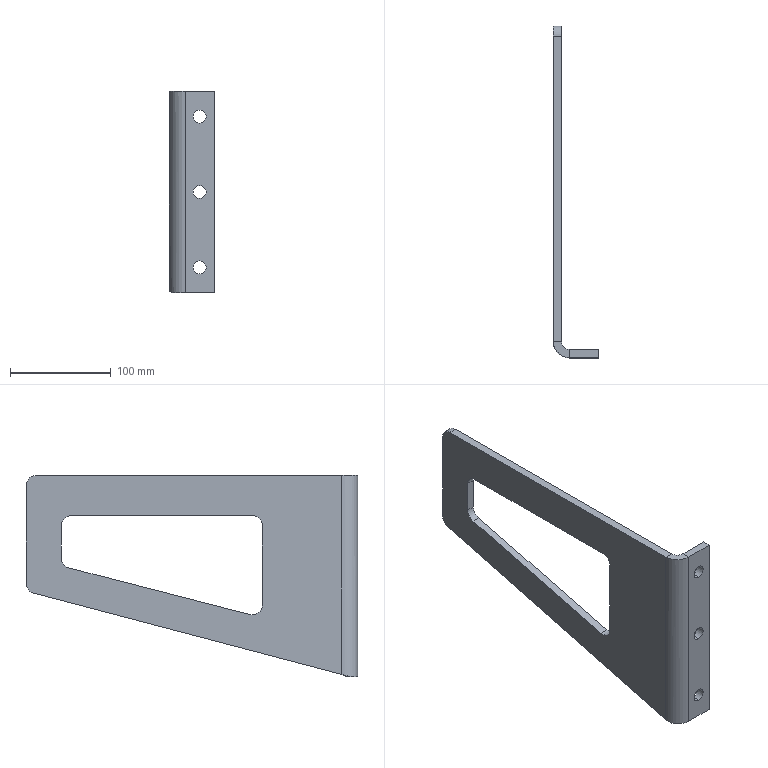Part | SolidWorks | features ICE 2, FlatPattern 1, SMBaseFlange 1, SheetMetal 1 | 1 solid | 31 faces | box 45 x 330 x 200 mm | volume 345586 mm3 | plane 16 | cylinder 14 | spline 1 | commonest cylinder face diameters 13 x6 20 x6 16 x1 32 x1
STEP:
#1=CARTESIAN_POINT('',(-3.464,-55.999,-168.5));
#2=VERTEX_POINT('',#1);
#3=CARTESIAN_POINT('',(-3.464,-55.999,-181.5));
#4=VERTEX_POINT('',#3);
#5=CARTESIAN_POINT('',(-3.464,-55.999,-175.));
#6=DIRECTION('',(0.,-1.,0.));
#7=DIRECTION('',(0.,0.,-1.));
#8=AXIS2_PLACEMENT_3D('',#5,#6,#7);
#9=CIRCLE('',#8,6.5);
#10=EDGE_CURVE('',#2,#4,#9,.T.);
#11=ORIENTED_EDGE('',*,*,#10,.F.);
#12=CARTESIAN_POINT('',(-3.464,-63.999,-168.5));
#13=VERTEX_POINT('',#12);
#14=CARTESIAN_POINT('',(-3.464,266.001,-168.5));
#15=DIRECTION('',(0.,-1.,0.));
#16=VECTOR('',#15,1000.);
#17=LINE('',#14,#16);
#18=EDGE_CURVE('',#2,#13,#17,.T.);
#19=ORIENTED_EDGE('',*,*,#18,.T.);
#20=CARTESIAN_POINT('',(-3.464,-63.999,-181.5));
#21=VERTEX_POINT('',#20);
#22=CARTESIAN_POINT('',(-3.464,-63.999,-175.));
#23=DIRECTION('',(0.,-1.,0.));
#24=DIRECTION('',(0.,0.,-1.));
#25=AXIS2_PLACEMENT_3D('',#22,#23,#24);
#26=CIRCLE('',#25,6.5);
#27=EDGE_CURVE('',#13,#21,#26,.T.);
#28=ORIENTED_EDGE('',*,*,#27,.T.);
#29=CARTESIAN_POINT('',(-3.464,266.001,-181.5));
#30=DIRECTION('',(0.,-1.,0.));
#31=VECTOR('',#30,1000.);
#32=LINE('',#29,#31);
#33=EDGE_CURVE('',#4,#21,#32,.T.);
#34=ORIENTED_EDGE('',*,*,#33,.F.);
#35=EDGE_LOOP('',(#11,#19,#28,#34));
#36=FACE_OUTER_BOUND('',#35,.T.);
#37=CARTESIAN_POINT('',(-3.464,266.001,-175.));
#38=DIRECTION('',(0.,-1.,0.));
#39=DIRECTION('',(0.,0.,-1.));
#40=AXIS2_PLACEMENT_3D('',#37,#38,#39);
#41=CYLINDRICAL_SURFACE('',#40,6.5);
#42=ADVANCED_FACE('',(#36),#41,.F.);
#43=CARTESIAN_POINT('',(-3.464,-55.999,-93.5));
#44=VERTEX_POINT('',#43);
#45=CARTESIAN_POINT('',(-3.464,-55.999,-106.5));
#46=VERTEX_POINT('',#45);
#47=CARTESIAN_POINT('',(-3.464,-55.999,-100.));
#48=DIRECTION('',(0.,-1.,0.));
#49=DIRECTION('',(0.,0.,-1.));
#50=AXIS2_PLACEMENT_3D('',#47,#48,#49);
#51=CIRCLE('',#50,6.5);
#52=EDGE_CURVE('',#44,#46,#51,.T.);
#53=ORIENTED_EDGE('',*,*,#52,.F.);
#54=CARTESIAN_POINT('',(-3.464,-63.999,-93.5));
#55=VERTEX_POINT('',#54);
#56=CARTESIAN_POINT('',(-3.464,266.001,-93.5));
#57=DIRECTION('',(0.,-1.,0.));
#58=VECTOR('',#57,1000.);
#59=LINE('',#56,#58);
#60=EDGE_CURVE('',#44,#55,#59,.T.);
#61=ORIENTED_EDGE('',*,*,#60,.T.);
#62=CARTESIAN_POINT('',(-3.464,-63.999,-106.5));
#63=VERTEX_POINT('',#62);
#64=CARTESIAN_POINT('',(-3.464,-63.999,-100.));
#65=DIRECTION('',(0.,-1.,0.));
#66=DIRECTION('',(0.,0.,-1.));
#67=AXIS2_PLACEMENT_3D('',#64,#65,#66);
#68=CIRCLE('',#67,6.5);
#69=EDGE_CURVE('',#55,#63,#68,.T.);
#70=ORIENTED_EDGE('',*,*,#69,.T.);
#71=CARTESIAN_POINT('',(-3.464,266.001,-106.5));
#72=DIRECTION('',(0.,-1.,0.));
#73=VECTOR('',#72,1000.);
#74=LINE('',#71,#73);
#75=EDGE_CURVE('',#46,#63,#74,.T.);
#76=ORIENTED_EDGE('',*,*,#75,.F.);
#77=EDGE_LOOP('',(#53,#61,#70,#76));
#78=FACE_OUTER_BOUND('',#77,.T.);
#79=CARTESIAN_POINT('',(-3.464,266.001,-100.));
#80=DIRECTION('',(0.,-1.,0.));
#81=DIRECTION('',(0.,0.,-1.));
#82=AXIS2_PLACEMENT_3D('',#79,#80,#81);
#83=CYLINDRICAL_SURFACE('',#82,6.5);
#84=ADVANCED_FACE('',(#78),#83,.F.);
#85=CARTESIAN_POINT('',(-3.465,-55.999,-18.5));
#86=VERTEX_POINT('',#85);
#87=CARTESIAN_POINT('',(-3.465,-55.999,-31.5));
#88=VERTEX_POINT('',#87);
#89=CARTESIAN_POINT('',(-3.465,-55.999,-25.));
#90=DIRECTION('',(0.,-1.,0.));
#91=DIRECTION('',(0.,0.,-1.));
#92=AXIS2_PLACEMENT_3D('',#89,#90,#91);
#93=CIRCLE('',#92,6.5);
#94=EDGE_CURVE('',#86,#88,#93,.T.);
#95=ORIENTED_EDGE('',*,*,#94,.F.);
#96=CARTESIAN_POINT('',(-3.465,-63.999,-18.5));
#97=VERTEX_POINT('',#96);
#98=CARTESIAN_POINT('',(-3.465,266.001,-18.5));
#99=DIRECTION('',(0.,-1.,0.));
#100=VECTOR('',#99,1000.);
#101=LINE('',#98,#100);
#102=EDGE_CURVE('',#86,#97,#101,.T.);
#103=ORIENTED_EDGE('',*,*,#102,.T.);
#104=CARTESIAN_POINT('',(-3.465,-63.999,-31.5));
#105=VERTEX_POINT('',#104);
#106=CARTESIAN_POINT('',(-3.465,-63.999,-25.));
#107=DIRECTION('',(0.,-1.,0.));
#108=DIRECTION('',(0.,0.,-1.));
#109=AXIS2_PLACEMENT_3D('',#106,#107,#108);
#110=CIRCLE('',#109,6.5);
#111=EDGE_CURVE('',#97,#105,#110,.T.);
#112=ORIENTED_EDGE('',*,*,#111,.T.);
#113=CARTESIAN_POINT('',(-3.465,266.001,-31.5));
#114=DIRECTION('',(0.,-1.,0.));
#115=VECTOR('',#114,1000.);
#116=LINE('',#113,#115);
#117=EDGE_CURVE('',#88,#105,#116,.T.);
#118=ORIENTED_EDGE('',*,*,#117,.F.);
#119=EDGE_LOOP('',(#95,#103,#112,#118));
#120=FACE_OUTER_BOUND('',#119,.T.);
#121=CARTESIAN_POINT('',(-3.465,266.001,-25.));
#122=DIRECTION('',(0.,-1.,0.));
#123=DIRECTION('',(0.,0.,-1.));
#124=AXIS2_PLACEMENT_3D('',#121,#122,#123);
#125=CYLINDRICAL_SURFACE('',#124,6.5);
#126=ADVANCED_FACE('',(#120),#125,.F.);
#127=CARTESIAN_POINT('',(-33.465,43.495,-138.283));
#128=VERTEX_POINT('',#127);
#129=CARTESIAN_POINT('',(-33.465,223.495,-91.933));
#130=VERTEX_POINT('',#129);
#131=CARTESIAN_POINT('',(-33.465,43.495,-138.283));
#132=DIRECTION('',(0.,0.9684,0.2494));
#133=VECTOR('',#132,1000.);
#134=LINE('',#131,#133);
#135=EDGE_CURVE('',#128,#130,#134,.T.);
#136=ORIENTED_EDGE('',*,*,#135,.T.);
#137=CARTESIAN_POINT('',(-33.465,231.001,-82.249));
#138=VERTEX_POINT('',#137);
#139=CARTESIAN_POINT('',(-33.465,221.001,-82.249));
#140=DIRECTION('',(1.,0.,0.));
#141=DIRECTION('',(0.,1.,0.));
#142=AXIS2_PLACEMENT_3D('',#139,#140,#141);
#143=CIRCLE('',#142,10.);
#144=EDGE_CURVE('',#130,#138,#143,.T.);
#145=ORIENTED_EDGE('',*,*,#144,.T.);
#146=CARTESIAN_POINT('',(-33.465,231.001,-50.));
#147=VERTEX_POINT('',#146);
#148=CARTESIAN_POINT('',(-33.465,231.001,-200.));
#149=DIRECTION('',(0.,0.,1.));
#150=VECTOR('',#149,1000.);
#151=LINE('',#148,#150);
#152=EDGE_CURVE('',#138,#147,#151,.T.);
#153=ORIENTED_EDGE('',*,*,#152,.T.);
#154=CARTESIAN_POINT('',(-33.465,221.001,-40.));
#155=VERTEX_POINT('',#154);
#156=CARTESIAN_POINT('',(-33.465,221.001,-50.));
#157=DIRECTION('',(1.,0.,0.));
#158=DIRECTION('',(0.,1.,0.));
#159=AXIS2_PLACEMENT_3D('',#156,#157,#158);
#160=CIRCLE('',#159,10.);
#161=EDGE_CURVE('',#147,#155,#160,.T.);
#162=ORIENTED_EDGE('',*,*,#161,.T.);
#163=CARTESIAN_POINT('',(-33.465,41.001,-40.));
#164=VERTEX_POINT('',#163);
#165=CARTESIAN_POINT('',(-33.465,266.001,-40.));
#166=DIRECTION('',(0.,-1.,0.));
#167=VECTOR('',#166,1000.);
#168=LINE('',#165,#167);
#169=EDGE_CURVE('',#155,#164,#168,.T.);
#170=ORIENTED_EDGE('',*,*,#169,.T.);
#171=CARTESIAN_POINT('',(-33.465,31.001,-50.));
#172=VERTEX_POINT('',#171);
#173=CARTESIAN_POINT('',(-33.465,41.001,-50.));
#174=DIRECTION('',(1.,0.,0.));
#175=DIRECTION('',(0.,1.,0.));
#176=AXIS2_PLACEMENT_3D('',#173,#174,#175);
#177=CIRCLE('',#176,10.);
#178=EDGE_CURVE('',#164,#172,#177,.T.);
#179=ORIENTED_EDGE('',*,*,#178,.T.);
#180=CARTESIAN_POINT('',(-33.465,31.001,-128.599));
#181=VERTEX_POINT('',#180);
#182=CARTESIAN_POINT('',(-33.465,31.001,-200.));
#183=DIRECTION('',(0.,0.,-1.));
#184=VECTOR('',#183,1000.);
#185=LINE('',#182,#184);
#186=EDGE_CURVE('',#172,#181,#185,.T.);
#187=ORIENTED_EDGE('',*,*,#186,.T.);
#188=CARTESIAN_POINT('',(-33.465,41.001,-128.599));
#189=DIRECTION('',(1.,0.,0.));
#190=DIRECTION('',(0.,1.,0.));
#191=AXIS2_PLACEMENT_3D('',#188,#189,#190);
#192=CIRCLE('',#191,10.);
#193=EDGE_CURVE('',#181,#128,#192,.T.);
#194=ORIENTED_EDGE('',*,*,#193,.T.);
#195=EDGE_LOOP('',(#136,#145,#153,#162,#170,#179,#187,#194));
#196=FACE_BOUND('',#195,.T.);
#197=CARTESIAN_POINT('',(-33.465,266.001,-107.297));
#198=VERTEX_POINT('',#197);
#199=CARTESIAN_POINT('',(-33.465,266.001,-10.));
#200=VERTEX_POINT('',#199);
#201=CARTESIAN_POINT('',(-33.465,266.001,-200.));
#202=DIRECTION('',(0.,0.,1.));
#203=VECTOR('',#202,1000.);
#204=LINE('',#201,#203);
#205=EDGE_CURVE('',#198,#200,#204,.T.);
#206=ORIENTED_EDGE('',*,*,#205,.F.);
#207=CARTESIAN_POINT('',(-33.465,258.553,-116.966));
#208=VERTEX_POINT('',#207);
#209=CARTESIAN_POINT('',(-33.465,256.001,-107.297));
#210=DIRECTION('',(-1.,0.,0.));
#211=DIRECTION('',(0.,-1.,0.));
#212=AXIS2_PLACEMENT_3D('',#209,#210,#211);
#213=CIRCLE('',#212,10.);
#214=EDGE_CURVE('',#198,#208,#213,.T.);
#215=ORIENTED_EDGE('',*,*,#214,.T.);
#216=CARTESIAN_POINT('',(-33.465,-47.999,-197.888));
#217=VERTEX_POINT('',#216);
#218=CARTESIAN_POINT('',(-33.465,-55.999,-200.));
#219=DIRECTION('',(0.,-0.9669,-0.2552));
#220=VECTOR('',#219,1000.);
#221=LINE('',#218,#220);
#222=EDGE_CURVE('',#208,#217,#221,.T.);
#223=ORIENTED_EDGE('',*,*,#222,.T.);
#224=CARTESIAN_POINT('',(-33.465,-47.999,0.));
#225=VERTEX_POINT('',#224);
#226=CARTESIAN_POINT('',(-33.465,-47.999,-200.));
#227=DIRECTION('',(0.,0.,1.));
#228=VECTOR('',#227,1000.);
#229=LINE('',#226,#228);
#230=EDGE_CURVE('',#217,#225,#229,.T.);
#231=ORIENTED_EDGE('',*,*,#230,.T.);
#232=CARTESIAN_POINT('',(-33.465,256.001,0.));
#233=VERTEX_POINT('',#232);
#234=CARTESIAN_POINT('',(-33.465,266.001,0.));
#235=DIRECTION('',(0.,-1.,0.));
#236=VECTOR('',#235,1000.);
#237=LINE('',#234,#236);
#238=EDGE_CURVE('',#233,#225,#237,.T.);
#239=ORIENTED_EDGE('',*,*,#238,.F.);
#240=CARTESIAN_POINT('',(-33.465,256.001,-10.));
#241=DIRECTION('',(-1.,0.,0.));
#242=DIRECTION('',(0.,-1.,0.));
#243=AXIS2_PLACEMENT_3D('',#240,#241,#242);
#244=CIRCLE('',#243,10.);
#245=EDGE_CURVE('',#233,#200,#244,.T.);
#246=ORIENTED_EDGE('',*,*,#245,.T.);
#247=EDGE_LOOP('',(#206,#215,#223,#231,#239,#246));
#248=FACE_OUTER_BOUND('',#247,.T.);
#249=CARTESIAN_POINT('',(-33.465,266.001,-200.));
#250=DIRECTION('',(-1.,0.,0.));
#251=DIRECTION('',(0.,-1.,0.));
#252=AXIS2_PLACEMENT_3D('',#249,#250,#251);
#253=PLANE('',#252);
#254=ADVANCED_FACE('',(#196,#248),#253,.T.);
#255=CARTESIAN_POINT('',(-25.465,223.495,-91.933));
#256=VERTEX_POINT('',#255);
#257=CARTESIAN_POINT('',(-25.465,231.001,-82.249));
#258=VERTEX_POINT('',#257);
#259=CARTESIAN_POINT('',(-25.465,221.001,-82.249));
#260=DIRECTION('',(1.,0.,0.));
#261=DIRECTION('',(0.,1.,0.));
#262=AXIS2_PLACEMENT_3D('',#259,#260,#261);
#263=CIRCLE('',#262,10.);
#264=EDGE_CURVE('',#256,#258,#263,.T.);
#265=ORIENTED_EDGE('',*,*,#264,.F.);
#266=CARTESIAN_POINT('',(-25.465,43.495,-138.283));
#267=VERTEX_POINT('',#266);
#268=CARTESIAN_POINT('',(-25.465,43.495,-138.283));
#269=DIRECTION('',(0.,0.9684,0.2494));
#270=VECTOR('',#269,1000.);
#271=LINE('',#268,#270);
#272=EDGE_CURVE('',#267,#256,#271,.T.);
#273=ORIENTED_EDGE('',*,*,#272,.F.);
#274=CARTESIAN_POINT('',(-25.465,31.001,-128.599));
#275=VERTEX_POINT('',#274);
#276=CARTESIAN_POINT('',(-25.465,41.001,-128.599));
#277=DIRECTION('',(1.,0.,0.));
#278=DIRECTION('',(0.,-1.,0.));
#279=AXIS2_PLACEMENT_3D('',#276,#277,#278);
#280=CIRCLE('',#279,10.);
#281=EDGE_CURVE('',#275,#267,#280,.T.);
#282=ORIENTED_EDGE('',*,*,#281,.F.);
#283=CARTESIAN_POINT('',(-25.465,31.001,-50.));
#284=VERTEX_POINT('',#283);
#285=CARTESIAN_POINT('',(-25.465,31.001,-50.));
#286=DIRECTION('',(0.,0.,-1.));
#287=VECTOR('',#286,1000.);
#288=LINE('',#285,#287);
#289=EDGE_CURVE('',#284,#275,#288,.T.);
#290=ORIENTED_EDGE('',*,*,#289,.F.);
#291=CARTESIAN_POINT('',(-25.465,41.001,-40.));
#292=VERTEX_POINT('',#291);
#293=CARTESIAN_POINT('',(-25.465,41.001,-50.));
#294=DIRECTION('',(1.,0.,0.));
#295=DIRECTION('',(0.,1.,0.));
#296=AXIS2_PLACEMENT_3D('',#293,#294,#295);
#297=CIRCLE('',#296,10.);
#298=EDGE_CURVE('',#292,#284,#297,.T.);
#299=ORIENTED_EDGE('',*,*,#298,.F.);
#300=CARTESIAN_POINT('',(-25.465,221.001,-40.));
#301=VERTEX_POINT('',#300);
#302=CARTESIAN_POINT('',(-25.465,41.001,-40.));
#303=DIRECTION('',(0.,-1.,0.));
#304=VECTOR('',#303,1000.);
#305=LINE('',#302,#304);
#306=EDGE_CURVE('',#301,#292,#305,.T.);
#307=ORIENTED_EDGE('',*,*,#306,.F.);
#308=CARTESIAN_POINT('',(-25.465,231.001,-50.));
#309=VERTEX_POINT('',#308);
#310=CARTESIAN_POINT('',(-25.465,221.001,-50.));
#311=DIRECTION('',(1.,0.,0.));
#312=DIRECTION('',(0.,-1.,0.));
#313=AXIS2_PLACEMENT_3D('',#310,#311,#312);
#314=CIRCLE('',#313,10.);
#315=EDGE_CURVE('',#309,#301,#314,.T.);
#316=ORIENTED_EDGE('',*,*,#315,.F.);
#317=CARTESIAN_POINT('',(-25.465,231.001,-50.));
#318=DIRECTION('',(0.,0.,1.));
#319=VECTOR('',#318,1000.);
#320=LINE('',#317,#319);
#321=EDGE_CURVE('',#258,#309,#320,.T.);
#322=ORIENTED_EDGE('',*,*,#321,.F.);
#323=EDGE_LOOP('',(#265,#273,#282,#290,#299,#307,#316,#322));
#324=FACE_BOUND('',#323,.T.);
#325=CARTESIAN_POINT('',(-25.465,266.001,-107.297));
#326=VERTEX_POINT('',#325);
#327=CARTESIAN_POINT('',(-25.465,258.553,-116.966));
#328=VERTEX_POINT('',#327);
#329=CARTESIAN_POINT('',(-25.465,256.001,-107.297));
#330=DIRECTION('',(-1.,0.,0.));
#331=DIRECTION('',(0.,1.,0.));
#332=AXIS2_PLACEMENT_3D('',#329,#330,#331);
#333=CIRCLE('',#332,10.);
#334=EDGE_CURVE('',#326,#328,#333,.T.);
#335=ORIENTED_EDGE('',*,*,#334,.F.);
#336=CARTESIAN_POINT('',(-25.465,266.001,-10.));
#337=VERTEX_POINT('',#336);
#338=CARTESIAN_POINT('',(-25.465,266.001,-200.));
#339=DIRECTION('',(0.,0.,1.));
#340=VECTOR('',#339,1000.);
#341=LINE('',#338,#340);
#342=EDGE_CURVE('',#326,#337,#341,.T.);
#343=ORIENTED_EDGE('',*,*,#342,.T.);
#344=CARTESIAN_POINT('',(-25.465,256.001,0.));
#345=VERTEX_POINT('',#344);
#346=CARTESIAN_POINT('',(-25.465,256.001,-10.));
#347=DIRECTION('',(-1.,0.,0.));
#348=DIRECTION('',(0.,-1.,0.));
#349=AXIS2_PLACEMENT_3D('',#346,#347,#348);
#350=CIRCLE('',#349,10.);
#351=EDGE_CURVE('',#345,#337,#350,.T.);
#352=ORIENTED_EDGE('',*,*,#351,.F.);
#353=CARTESIAN_POINT('',(-25.465,-47.999,0.));
#354=VERTEX_POINT('',#353);
#355=CARTESIAN_POINT('',(-25.465,266.001,0.));
#356=DIRECTION('',(0.,-1.,0.));
#357=VECTOR('',#356,1000.);
#358=LINE('',#355,#357);
#359=EDGE_CURVE('',#345,#354,#358,.T.);
#360=ORIENTED_EDGE('',*,*,#359,.T.);
#361=CARTESIAN_POINT('',(-25.465,-47.999,-197.888));
#362=VERTEX_POINT('',#361);
#363=CARTESIAN_POINT('',(-25.465,-47.999,-200.));
#364=DIRECTION('',(0.,0.,1.));
#365=VECTOR('',#364,1000.);
#366=LINE('',#363,#365);
#367=EDGE_CURVE('',#362,#354,#366,.T.);
#368=ORIENTED_EDGE('',*,*,#367,.F.);
#369=CARTESIAN_POINT('',(-25.465,-55.999,-200.));
#370=DIRECTION('',(0.,-0.9669,-0.2552));
#371=VECTOR('',#370,1000.);
#372=LINE('',#369,#371);
#373=EDGE_CURVE('',#328,#362,#372,.T.);
#374=ORIENTED_EDGE('',*,*,#373,.F.);
#375=EDGE_LOOP('',(#335,#343,#352,#360,#368,#374));
#376=FACE_OUTER_BOUND('',#375,.T.);
#377=CARTESIAN_POINT('',(-25.465,266.001,-200.));
#378=DIRECTION('',(-1.,0.,0.));
#379=DIRECTION('',(0.,-1.,0.));
#380=AXIS2_PLACEMENT_3D('',#377,#378,#379);
#381=PLANE('',#380);
#382=ADVANCED_FACE('',(#324,#376),#381,.F.);
#383=CARTESIAN_POINT('',(-31.321,-55.999,-200.));
#384=VERTEX_POINT('',#383);
#385=CARTESIAN_POINT('',(-17.465,-63.999,-200.));
#386=VERTEX_POINT('',#385);
#387=CARTESIAN_POINT('',(-17.465,-47.999,-200.));
#388=DIRECTION('',(0.,0.,1.));
#389=DIRECTION('',(-1.,0.,0.));
#390=AXIS2_PLACEMENT_3D('',#387,#388,#389);
#391=CIRCLE('',#390,16.);
#392=EDGE_CURVE('',#384,#386,#391,.T.);
#393=ORIENTED_EDGE('',*,*,#392,.F.);
#394=CARTESIAN_POINT('',(-24.393,-51.999,-200.));
#395=VERTEX_POINT('',#394);
#396=CARTESIAN_POINT('',(-31.321,-55.999,-200.));
#397=DIRECTION('',(0.866,0.5,0.));
#398=VECTOR('',#397,1000.);
#399=LINE('',#396,#398);
#400=EDGE_CURVE('',#384,#395,#399,.T.);
#401=ORIENTED_EDGE('',*,*,#400,.T.);
#402=CARTESIAN_POINT('',(-17.465,-55.999,-200.));
#403=VERTEX_POINT('',#402);
#404=CARTESIAN_POINT('',(-17.465,-47.999,-200.));
#405=DIRECTION('',(0.,0.,1.));
#406=DIRECTION('',(1.,0.,0.));
#407=AXIS2_PLACEMENT_3D('',#404,#405,#406);
#408=CIRCLE('',#407,8.);
#409=EDGE_CURVE('',#395,#403,#408,.T.);
#410=ORIENTED_EDGE('',*,*,#409,.T.);
#411=CARTESIAN_POINT('',(-17.465,-63.999,-200.));
#412=DIRECTION('',(0.,1.,0.));
#413=VECTOR('',#412,1000.);
#414=LINE('',#411,#413);
#415=EDGE_CURVE('',#386,#403,#414,.T.);
#416=ORIENTED_EDGE('',*,*,#415,.F.);
#417=EDGE_LOOP('',(#393,#401,#410,#416));
#418=FACE_OUTER_BOUND('',#417,.T.);
#419=CARTESIAN_POINT('',(-17.465,-63.999,-200.));
#420=DIRECTION('',(0.,0.,-1.));
#421=DIRECTION('',(-1.,0.,0.));
#422=AXIS2_PLACEMENT_3D('',#419,#420,#421);
#423=PLANE('',#422);
#424=ADVANCED_FACE('',(#418),#423,.T.);
#425=ORIENTED_EDGE('',*,*,#230,.F.);
#426=CARTESIAN_POINT('',(-31.321,-55.999,-200.));
#427=CARTESIAN_POINT('',(-32.733,-53.552,-199.354));
#428=CARTESIAN_POINT('',(-33.465,-50.824,-198.634));
#429=CARTESIAN_POINT('',(-33.465,-47.999,-197.888));
#430=(BOUNDED_CURVE()B_SPLINE_CURVE(3,(#426,#427,#428,#429),.UNSPECIFIED.,.F.,.T.)B_SPLINE_CURVE_WITH_KNOTS((4,4),(4.189,4.712),.UNSPECIFIED.)CURVE()GEOMETRIC_REPRESENTATION_ITEM()RATIONAL_B_SPLINE_CURVE((1.,0.9773,0.9773,1.))REPRESENTATION_ITEM(''));
#431=EDGE_CURVE('',#384,#217,#430,.T.);
#432=ORIENTED_EDGE('',*,*,#431,.F.);
#433=ORIENTED_EDGE('',*,*,#392,.T.);
#434=CARTESIAN_POINT('',(-17.465,-63.999,0.));
#435=VERTEX_POINT('',#434);
#436=CARTESIAN_POINT('',(-17.465,-63.999,-200.));
#437=DIRECTION('',(0.,0.,1.));
#438=VECTOR('',#437,1000.);
#439=LINE('',#436,#438);
#440=EDGE_CURVE('',#386,#435,#439,.T.);
#441=ORIENTED_EDGE('',*,*,#440,.T.);
#442=CARTESIAN_POINT('',(-17.465,-47.999,0.));
#443=DIRECTION('',(0.,0.,1.));
#444=DIRECTION('',(-1.,0.,0.));
#445=AXIS2_PLACEMENT_3D('',#442,#443,#444);
#446=CIRCLE('',#445,16.);
#447=EDGE_CURVE('',#225,#435,#446,.T.);
#448=ORIENTED_EDGE('',*,*,#447,.F.);
#449=EDGE_LOOP('',(#425,#432,#433,#441,#448));
#450=FACE_OUTER_BOUND('',#449,.T.);
#451=CARTESIAN_POINT('',(-17.465,-47.999,-200.));
#452=DIRECTION('',(0.,0.,1.));
#453=DIRECTION('',(1.,0.,0.));
#454=AXIS2_PLACEMENT_3D('',#451,#452,#453);
#455=CYLINDRICAL_SURFACE('',#454,16.);
#456=ADVANCED_FACE('',(#450),#455,.T.);
#457=CARTESIAN_POINT('',(-24.393,-51.999,-200.));
#458=CARTESIAN_POINT('',(-25.099,-50.776,-199.354));
#459=CARTESIAN_POINT('',(-25.465,-49.411,-198.634));
#460=CARTESIAN_POINT('',(-25.465,-47.999,-197.888));
#461=(BOUNDED_CURVE()B_SPLINE_CURVE(3,(#457,#458,#459,#460),.UNSPECIFIED.,.F.,.T.)B_SPLINE_CURVE_WITH_KNOTS((4,4),(4.189,4.712),.UNSPECIFIED.)CURVE()GEOMETRIC_REPRESENTATION_ITEM()RATIONAL_B_SPLINE_CURVE((1.,0.9773,0.9773,1.))REPRESENTATION_ITEM(''));
#462=EDGE_CURVE('',#395,#362,#461,.T.);
#463=ORIENTED_EDGE('',*,*,#462,.T.);
#464=ORIENTED_EDGE('',*,*,#367,.T.);
#465=CARTESIAN_POINT('',(-17.465,-55.999,0.));
#466=VERTEX_POINT('',#465);
#467=CARTESIAN_POINT('',(-17.465,-47.999,0.));
#468=DIRECTION('',(0.,0.,1.));
#469=DIRECTION('',(1.,0.,0.));
#470=AXIS2_PLACEMENT_3D('',#467,#468,#469);
#471=CIRCLE('',#470,8.);
#472=EDGE_CURVE('',#354,#466,#471,.T.);
#473=ORIENTED_EDGE('',*,*,#472,.T.);
#474=CARTESIAN_POINT('',(-17.465,-55.999,-200.));
#475=DIRECTION('',(0.,0.,1.));
#476=VECTOR('',#475,1000.);
#477=LINE('',#474,#476);
#478=EDGE_CURVE('',#403,#466,#477,.T.);
#479=ORIENTED_EDGE('',*,*,#478,.F.);
#480=ORIENTED_EDGE('',*,*,#409,.F.);
#481=EDGE_LOOP('',(#463,#464,#473,#479,#480));
#482=FACE_OUTER_BOUND('',#481,.T.);
#483=CARTESIAN_POINT('',(-17.465,-47.999,-200.));
#484=DIRECTION('',(0.,0.,1.));
#485=DIRECTION('',(1.,0.,0.));
#486=AXIS2_PLACEMENT_3D('',#483,#484,#485);
#487=CYLINDRICAL_SURFACE('',#486,8.);
#488=ADVANCED_FACE('',(#482),#487,.F.);
#489=ORIENTED_EDGE('',*,*,#359,.F.);
#490=CARTESIAN_POINT('',(-25.465,256.001,0.));
#491=DIRECTION('',(-1.,0.,0.));
#492=VECTOR('',#491,1000.);
#493=LINE('',#490,#492);
#494=EDGE_CURVE('',#345,#233,#493,.T.);
#495=ORIENTED_EDGE('',*,*,#494,.T.);
#496=ORIENTED_EDGE('',*,*,#238,.T.);
#497=CARTESIAN_POINT('',(-33.465,-47.999,0.));
#498=DIRECTION('',(1.,0.,0.));
#499=VECTOR('',#498,1000.);
#500=LINE('',#497,#499);
#501=EDGE_CURVE('',#225,#354,#500,.T.);
#502=ORIENTED_EDGE('',*,*,#501,.T.);
#503=EDGE_LOOP('',(#489,#495,#496,#502));
#504=FACE_OUTER_BOUND('',#503,.T.);
#505=CARTESIAN_POINT('',(-17.465,-55.999,0.));
#506=DIRECTION('',(0.,0.,1.));
#507=DIRECTION('',(1.,0.,0.));
#508=AXIS2_PLACEMENT_3D('',#505,#506,#507);
#509=PLANE('',#508);
#510=ADVANCED_FACE('',(#504),#509,.T.);
#511=ORIENTED_EDGE('',*,*,#342,.F.);
#512=CARTESIAN_POINT('',(-25.465,266.001,-107.297));
#513=DIRECTION('',(-1.,0.,0.));
#514=VECTOR('',#513,1000.);
#515=LINE('',#512,#514);
#516=EDGE_CURVE('',#326,#198,#515,.T.);
#517=ORIENTED_EDGE('',*,*,#516,.T.);
#518=ORIENTED_EDGE('',*,*,#205,.T.);
#519=CARTESIAN_POINT('',(-25.465,266.001,-10.));
#520=DIRECTION('',(-1.,0.,0.));
#521=VECTOR('',#520,1000.);
#522=LINE('',#519,#521);
#523=EDGE_CURVE('',#337,#200,#522,.T.);
#524=ORIENTED_EDGE('',*,*,#523,.F.);
#525=EDGE_LOOP('',(#511,#517,#518,#524));
#526=FACE_OUTER_BOUND('',#525,.T.);
#527=CARTESIAN_POINT('',(-33.465,266.001,-200.));
#528=DIRECTION('',(0.,-1.,0.));
#529=DIRECTION('',(0.,0.,-1.));
#530=AXIS2_PLACEMENT_3D('',#527,#528,#529);
#531=PLANE('',#530);
#532=ADVANCED_FACE('',(#526),#531,.F.);
#533=CARTESIAN_POINT('',(11.535,-63.999,-200.));
#534=VERTEX_POINT('',#533);
#535=CARTESIAN_POINT('',(-33.465,-63.999,-200.));
#536=DIRECTION('',(1.,0.,0.));
#537=VECTOR('',#536,1000.);
#538=LINE('',#535,#537);
#539=EDGE_CURVE('',#386,#534,#538,.T.);
#540=ORIENTED_EDGE('',*,*,#539,.F.);
#541=ORIENTED_EDGE('',*,*,#415,.T.);
#542=CARTESIAN_POINT('',(11.535,-55.999,-200.));
#543=VERTEX_POINT('',#542);
#544=CARTESIAN_POINT('',(-33.465,-55.999,-200.));
#545=DIRECTION('',(1.,0.,0.));
#546=VECTOR('',#545,1000.);
#547=LINE('',#544,#546);
#548=EDGE_CURVE('',#403,#543,#547,.T.);
#549=ORIENTED_EDGE('',*,*,#548,.T.);
#550=CARTESIAN_POINT('',(11.535,-55.999,-200.));
#551=DIRECTION('',(0.,-1.,0.));
#552=VECTOR('',#551,1000.);
#553=LINE('',#550,#552);
#554=EDGE_CURVE('',#543,#534,#553,.T.);
#555=ORIENTED_EDGE('',*,*,#554,.T.);
#556=EDGE_LOOP('',(#540,#541,#549,#555));
#557=FACE_OUTER_BOUND('',#556,.T.);
#558=CARTESIAN_POINT('',(-25.465,-47.999,-200.));
#559=DIRECTION('',(0.,0.,-1.));
#560=DIRECTION('',(-1.,0.,0.));
#561=AXIS2_PLACEMENT_3D('',#558,#559,#560);
#562=PLANE('',#561);
#563=ADVANCED_FACE('',(#557),#562,.T.);
#564=ORIENTED_EDGE('',*,*,#501,.F.);
#565=ORIENTED_EDGE('',*,*,#447,.T.);
#566=CARTESIAN_POINT('',(-17.465,-55.999,0.));
#567=DIRECTION('',(0.,-1.,0.));
#568=VECTOR('',#567,1000.);
#569=LINE('',#566,#568);
#570=EDGE_CURVE('',#466,#435,#569,.T.);
#571=ORIENTED_EDGE('',*,*,#570,.F.);
#572=ORIENTED_EDGE('',*,*,#472,.F.);
#573=EDGE_LOOP('',(#564,#565,#571,#572));
#574=FACE_OUTER_BOUND('',#573,.T.);
#575=CARTESIAN_POINT('',(-33.465,-47.999,0.));
#576=DIRECTION('',(0.,0.,1.));
#577=DIRECTION('',(1.,0.,0.));
#578=AXIS2_PLACEMENT_3D('',#575,#576,#577);
#579=PLANE('',#578);
#580=ADVANCED_FACE('',(#574),#579,.T.);
#581=CARTESIAN_POINT('',(-3.464,-63.999,-175.));
#582=DIRECTION('',(0.,-1.,0.));
#583=DIRECTION('',(0.,0.,-1.));
#584=AXIS2_PLACEMENT_3D('',#581,#582,#583);
#585=CIRCLE('',#584,6.5);
#586=EDGE_CURVE('',#21,#13,#585,.T.);
#587=ORIENTED_EDGE('',*,*,#586,.F.);
#588=ORIENTED_EDGE('',*,*,#27,.F.);
#589=EDGE_LOOP('',(#587,#588));
#590=FACE_BOUND('',#589,.T.);
#591=CARTESIAN_POINT('',(-3.464,-63.999,-100.));
#592=DIRECTION('',(0.,-1.,0.));
#593=DIRECTION('',(0.,0.,-1.));
#594=AXIS2_PLACEMENT_3D('',#591,#592,#593);
#595=CIRCLE('',#594,6.5);
#596=EDGE_CURVE('',#63,#55,#595,.T.);
#597=ORIENTED_EDGE('',*,*,#596,.F.);
#598=ORIENTED_EDGE('',*,*,#69,.F.);
#599=EDGE_LOOP('',(#597,#598));
#600=FACE_BOUND('',#599,.T.);
#601=CARTESIAN_POINT('',(-3.465,-63.999,-25.));
#602=DIRECTION('',(0.,-1.,0.));
#603=DIRECTION('',(0.,0.,-1.));
#604=AXIS2_PLACEMENT_3D('',#601,#602,#603);
#605=CIRCLE('',#604,6.5);
#606=EDGE_CURVE('',#105,#97,#605,.T.);
#607=ORIENTED_EDGE('',*,*,#606,.F.);
#608=ORIENTED_EDGE('',*,*,#111,.F.);
#609=EDGE_LOOP('',(#607,#608));
#610=FACE_BOUND('',#609,.T.);
#611=CARTESIAN_POINT('',(11.535,-63.999,0.));
#612=VERTEX_POINT('',#611);
#613=CARTESIAN_POINT('',(-33.465,-63.999,0.));
#614=DIRECTION('',(1.,0.,0.));
#615=VECTOR('',#614,1000.);
#616=LINE('',#613,#615);
#617=EDGE_CURVE('',#435,#612,#616,.T.);
#618=ORIENTED_EDGE('',*,*,#617,.F.);
#619=ORIENTED_EDGE('',*,*,#440,.F.);
#620=ORIENTED_EDGE('',*,*,#539,.T.);
#621=CARTESIAN_POINT('',(11.535,-63.999,-200.));
#622=DIRECTION('',(0.,0.,1.));
#623=VECTOR('',#622,1000.);
#624=LINE('',#621,#623);
#625=EDGE_CURVE('',#534,#612,#624,.T.);
#626=ORIENTED_EDGE('',*,*,#625,.T.);
#627=EDGE_LOOP('',(#618,#619,#620,#626));
#628=FACE_OUTER_BOUND('',#627,.T.);
#629=CARTESIAN_POINT('',(-33.465,-63.999,-200.));
#630=DIRECTION('',(0.,-1.,0.));
#631=DIRECTION('',(0.,0.,-1.));
#632=AXIS2_PLACEMENT_3D('',#629,#630,#631);
#633=PLANE('',#632);
#634=ADVANCED_FACE('',(#590,#600,#610,#628),#633,.T.);
#635=CARTESIAN_POINT('',(-3.464,-55.999,-175.));
#636=DIRECTION('',(0.,-1.,0.));
#637=DIRECTION('',(0.,0.,-1.));
#638=AXIS2_PLACEMENT_3D('',#635,#636,#637);
#639=CIRCLE('',#638,6.5);
#640=EDGE_CURVE('',#4,#2,#639,.T.);
#641=ORIENTED_EDGE('',*,*,#640,.T.);
#642=ORIENTED_EDGE('',*,*,#10,.T.);
#643=EDGE_LOOP('',(#641,#642));
#644=FACE_BOUND('',#643,.T.);
#645=CARTESIAN_POINT('',(-3.464,-55.999,-100.));
#646=DIRECTION('',(0.,-1.,0.));
#647=DIRECTION('',(0.,0.,-1.));
#648=AXIS2_PLACEMENT_3D('',#645,#646,#647);
#649=CIRCLE('',#648,6.5);
#650=EDGE_CURVE('',#46,#44,#649,.T.);
#651=ORIENTED_EDGE('',*,*,#650,.T.);
#652=ORIENTED_EDGE('',*,*,#52,.T.);
#653=EDGE_LOOP('',(#651,#652));
#654=FACE_BOUND('',#653,.T.);
#655=CARTESIAN_POINT('',(-3.465,-55.999,-25.));
#656=DIRECTION('',(0.,-1.,0.));
#657=DIRECTION('',(0.,0.,-1.));
#658=AXIS2_PLACEMENT_3D('',#655,#656,#657);
#659=CIRCLE('',#658,6.5);
#660=EDGE_CURVE('',#88,#86,#659,.T.);
#661=ORIENTED_EDGE('',*,*,#660,.T.);
#662=ORIENTED_EDGE('',*,*,#94,.T.);
#663=EDGE_LOOP('',(#661,#662));
#664=FACE_BOUND('',#663,.T.);
#665=CARTESIAN_POINT('',(11.535,-55.999,0.));
#666=VERTEX_POINT('',#665);
#667=CARTESIAN_POINT('',(-33.465,-55.999,0.));
#668=DIRECTION('',(1.,0.,0.));
#669=VECTOR('',#668,1000.);
#670=LINE('',#667,#669);
#671=EDGE_CURVE('',#466,#666,#670,.T.);
#672=ORIENTED_EDGE('',*,*,#671,.T.);
#673=CARTESIAN_POINT('',(11.535,-55.999,-200.));
#674=DIRECTION('',(0.,0.,1.));
#675=VECTOR('',#674,1000.);
#676=LINE('',#673,#675);
#677=EDGE_CURVE('',#543,#666,#676,.T.);
#678=ORIENTED_EDGE('',*,*,#677,.F.);
#679=ORIENTED_EDGE('',*,*,#548,.F.);
#680=ORIENTED_EDGE('',*,*,#478,.T.);
#681=EDGE_LOOP('',(#672,#678,#679,#680));
#682=FACE_OUTER_BOUND('',#681,.T.);
#683=CARTESIAN_POINT('',(-33.465,-55.999,-200.));
#684=DIRECTION('',(0.,-1.,0.));
#685=DIRECTION('',(0.,0.,-1.));
#686=AXIS2_PLACEMENT_3D('',#683,#684,#685);
#687=PLANE('',#686);
#688=ADVANCED_FACE('',(#644,#654,#664,#682),#687,.F.);
#689=CARTESIAN_POINT('',(11.535,-55.999,0.));
#690=DIRECTION('',(0.,-1.,0.));
#691=VECTOR('',#690,1000.);
#692=LINE('',#689,#691);
#693=EDGE_CURVE('',#666,#612,#692,.T.);
#694=ORIENTED_EDGE('',*,*,#693,.T.);
#695=ORIENTED_EDGE('',*,*,#625,.F.);
#696=ORIENTED_EDGE('',*,*,#554,.F.);
#697=ORIENTED_EDGE('',*,*,#677,.T.);
#698=EDGE_LOOP('',(#694,#695,#696,#697));
#699=FACE_OUTER_BOUND('',#698,.T.);
#700=CARTESIAN_POINT('',(11.535,-55.999,-200.));
#701=DIRECTION('',(-1.,0.,0.));
#702=DIRECTION('',(0.,0.,1.));
#703=AXIS2_PLACEMENT_3D('',#700,#701,#702);
#704=PLANE('',#703);
#705=ADVANCED_FACE('',(#699),#704,.F.);
#706=ORIENTED_EDGE('',*,*,#617,.T.);
#707=ORIENTED_EDGE('',*,*,#693,.F.);
#708=ORIENTED_EDGE('',*,*,#671,.F.);
#709=ORIENTED_EDGE('',*,*,#570,.T.);
#710=EDGE_LOOP('',(#706,#707,#708,#709));
#711=FACE_OUTER_BOUND('',#710,.T.);
#712=CARTESIAN_POINT('',(-17.465,-47.999,0.));
#713=DIRECTION('',(0.,0.,1.));
#714=DIRECTION('',(1.,0.,0.));
#715=AXIS2_PLACEMENT_3D('',#712,#713,#714);
#716=PLANE('',#715);
#717=ADVANCED_FACE('',(#711),#716,.T.);
#718=ORIENTED_EDGE('',*,*,#494,.F.);
#719=ORIENTED_EDGE('',*,*,#351,.T.);
#720=ORIENTED_EDGE('',*,*,#523,.T.);
#721=ORIENTED_EDGE('',*,*,#245,.F.);
#722=EDGE_LOOP('',(#718,#719,#720,#721));
#723=FACE_OUTER_BOUND('',#722,.T.);
#724=CARTESIAN_POINT('',(-25.465,256.001,-10.));
#725=DIRECTION('',(-1.,0.,0.));
#726=DIRECTION('',(0.,-1.,0.));
#727=AXIS2_PLACEMENT_3D('',#724,#725,#726);
#728=CYLINDRICAL_SURFACE('',#727,10.);
#729=ADVANCED_FACE('',(#723),#728,.T.);
#730=CARTESIAN_POINT('',(-25.465,223.495,-91.933));
#731=DIRECTION('',(-1.,0.,0.));
#732=VECTOR('',#731,1000.);
#733=LINE('',#730,#732);
#734=EDGE_CURVE('',#256,#130,#733,.T.);
#735=ORIENTED_EDGE('',*,*,#734,.F.);
#736=ORIENTED_EDGE('',*,*,#264,.T.);
#737=CARTESIAN_POINT('',(-25.465,231.001,-82.249));
#738=DIRECTION('',(-1.,0.,0.));
#739=VECTOR('',#738,1000.);
#740=LINE('',#737,#739);
#741=EDGE_CURVE('',#258,#138,#740,.T.);
#742=ORIENTED_EDGE('',*,*,#741,.T.);
#743=ORIENTED_EDGE('',*,*,#144,.F.);
#744=EDGE_LOOP('',(#735,#736,#742,#743));
#745=FACE_OUTER_BOUND('',#744,.T.);
#746=CARTESIAN_POINT('',(-25.465,221.001,-82.249));
#747=DIRECTION('',(1.,0.,0.));
#748=DIRECTION('',(0.,1.,0.));
#749=AXIS2_PLACEMENT_3D('',#746,#747,#748);
#750=CYLINDRICAL_SURFACE('',#749,10.);
#751=ADVANCED_FACE('',(#745),#750,.F.);
#752=ORIENTED_EDGE('',*,*,#741,.F.);
#753=ORIENTED_EDGE('',*,*,#321,.T.);
#754=CARTESIAN_POINT('',(-25.465,231.001,-50.));
#755=DIRECTION('',(-1.,0.,0.));
#756=VECTOR('',#755,1000.);
#757=LINE('',#754,#756);
#758=EDGE_CURVE('',#309,#147,#757,.T.);
#759=ORIENTED_EDGE('',*,*,#758,.T.);
#760=ORIENTED_EDGE('',*,*,#152,.F.);
#761=EDGE_LOOP('',(#752,#753,#759,#760));
#762=FACE_OUTER_BOUND('',#761,.T.);
#763=CARTESIAN_POINT('',(-25.465,231.001,-50.));
#764=DIRECTION('',(0.,-1.,0.));
#765=DIRECTION('',(0.,0.,1.));
#766=AXIS2_PLACEMENT_3D('',#763,#764,#765);
#767=PLANE('',#766);
#768=ADVANCED_FACE('',(#762),#767,.T.);
#769=ORIENTED_EDGE('',*,*,#758,.F.);
#770=ORIENTED_EDGE('',*,*,#315,.T.);
#771=CARTESIAN_POINT('',(-25.465,221.001,-40.));
#772=DIRECTION('',(-1.,0.,0.));
#773=VECTOR('',#772,1000.);
#774=LINE('',#771,#773);
#775=EDGE_CURVE('',#301,#155,#774,.T.);
#776=ORIENTED_EDGE('',*,*,#775,.T.);
#777=ORIENTED_EDGE('',*,*,#161,.F.);
#778=EDGE_LOOP('',(#769,#770,#776,#777));
#779=FACE_OUTER_BOUND('',#778,.T.);
#780=CARTESIAN_POINT('',(-25.465,221.001,-50.));
#781=DIRECTION('',(1.,0.,0.));
#782=DIRECTION('',(0.,1.,0.));
#783=AXIS2_PLACEMENT_3D('',#780,#781,#782);
#784=CYLINDRICAL_SURFACE('',#783,10.);
#785=ADVANCED_FACE('',(#779),#784,.F.);
#786=ORIENTED_EDGE('',*,*,#775,.F.);
#787=ORIENTED_EDGE('',*,*,#306,.T.);
#788=CARTESIAN_POINT('',(-25.465,41.001,-40.));
#789=DIRECTION('',(-1.,0.,0.));
#790=VECTOR('',#789,1000.);
#791=LINE('',#788,#790);
#792=EDGE_CURVE('',#292,#164,#791,.T.);
#793=ORIENTED_EDGE('',*,*,#792,.T.);
#794=ORIENTED_EDGE('',*,*,#169,.F.);
#795=EDGE_LOOP('',(#786,#787,#793,#794));
#796=FACE_OUTER_BOUND('',#795,.T.);
#797=CARTESIAN_POINT('',(-25.465,41.001,-40.));
#798=DIRECTION('',(0.,0.,-1.));
#799=DIRECTION('',(0.,-1.,0.));
#800=AXIS2_PLACEMENT_3D('',#797,#798,#799);
#801=PLANE('',#800);
#802=ADVANCED_FACE('',(#796),#801,.T.);
#803=ORIENTED_EDGE('',*,*,#792,.F.);
#804=ORIENTED_EDGE('',*,*,#298,.T.);
#805=CARTESIAN_POINT('',(-25.465,31.001,-50.));
#806=DIRECTION('',(-1.,0.,0.));
#807=VECTOR('',#806,1000.);
#808=LINE('',#805,#807);
#809=EDGE_CURVE('',#284,#172,#808,.T.);
#810=ORIENTED_EDGE('',*,*,#809,.T.);
#811=ORIENTED_EDGE('',*,*,#178,.F.);
#812=EDGE_LOOP('',(#803,#804,#810,#811));
#813=FACE_OUTER_BOUND('',#812,.T.);
#814=CARTESIAN_POINT('',(-25.465,41.001,-50.));
#815=DIRECTION('',(1.,0.,0.));
#816=DIRECTION('',(0.,1.,0.));
#817=AXIS2_PLACEMENT_3D('',#814,#815,#816);
#818=CYLINDRICAL_SURFACE('',#817,10.);
#819=ADVANCED_FACE('',(#813),#818,.F.);
#820=ORIENTED_EDGE('',*,*,#809,.F.);
#821=ORIENTED_EDGE('',*,*,#289,.T.);
#822=CARTESIAN_POINT('',(-25.465,31.001,-128.599));
#823=DIRECTION('',(-1.,0.,0.));
#824=VECTOR('',#823,1000.);
#825=LINE('',#822,#824);
#826=EDGE_CURVE('',#275,#181,#825,.T.);
#827=ORIENTED_EDGE('',*,*,#826,.T.);
#828=ORIENTED_EDGE('',*,*,#186,.F.);
#829=EDGE_LOOP('',(#820,#821,#827,#828));
#830=FACE_OUTER_BOUND('',#829,.T.);
#831=CARTESIAN_POINT('',(-25.465,31.001,-50.));
#832=DIRECTION('',(0.,1.,0.));
#833=DIRECTION('',(0.,0.,-1.));
#834=AXIS2_PLACEMENT_3D('',#831,#832,#833);
#835=PLANE('',#834);
#836=ADVANCED_FACE('',(#830),#835,.T.);
#837=ORIENTED_EDGE('',*,*,#826,.F.);
#838=ORIENTED_EDGE('',*,*,#281,.T.);
#839=CARTESIAN_POINT('',(-25.465,43.495,-138.283));
#840=DIRECTION('',(-1.,0.,0.));
#841=VECTOR('',#840,1000.);
#842=LINE('',#839,#841);
#843=EDGE_CURVE('',#267,#128,#842,.T.);
#844=ORIENTED_EDGE('',*,*,#843,.T.);
#845=ORIENTED_EDGE('',*,*,#193,.F.);
#846=EDGE_LOOP('',(#837,#838,#844,#845));
#847=FACE_OUTER_BOUND('',#846,.T.);
#848=CARTESIAN_POINT('',(-25.465,41.001,-128.599));
#849=DIRECTION('',(1.,0.,0.));
#850=DIRECTION('',(0.,1.,0.));
#851=AXIS2_PLACEMENT_3D('',#848,#849,#850);
#852=CYLINDRICAL_SURFACE('',#851,10.);
#853=ADVANCED_FACE('',(#847),#852,.F.);
#854=ORIENTED_EDGE('',*,*,#272,.T.);
#855=ORIENTED_EDGE('',*,*,#734,.T.);
#856=ORIENTED_EDGE('',*,*,#135,.F.);
#857=ORIENTED_EDGE('',*,*,#843,.F.);
#858=EDGE_LOOP('',(#854,#855,#856,#857));
#859=FACE_OUTER_BOUND('',#858,.T.);
#860=CARTESIAN_POINT('',(-25.465,43.495,-138.283));
#861=DIRECTION('',(0.,-0.2494,0.9684));
#862=DIRECTION('',(0.,0.9684,0.2494));
#863=AXIS2_PLACEMENT_3D('',#860,#861,#862);
#864=PLANE('',#863);
#865=ADVANCED_FACE('',(#859),#864,.T.);
#866=ORIENTED_EDGE('',*,*,#516,.F.);
#867=ORIENTED_EDGE('',*,*,#334,.T.);
#868=CARTESIAN_POINT('',(-25.465,258.553,-116.966));
#869=DIRECTION('',(-1.,0.,0.));
#870=VECTOR('',#869,1000.);
#871=LINE('',#868,#870);
#872=EDGE_CURVE('',#328,#208,#871,.T.);
#873=ORIENTED_EDGE('',*,*,#872,.T.);
#874=ORIENTED_EDGE('',*,*,#214,.F.);
#875=EDGE_LOOP('',(#866,#867,#873,#874));
#876=FACE_OUTER_BOUND('',#875,.T.);
#877=CARTESIAN_POINT('',(-25.465,256.001,-107.297));
#878=DIRECTION('',(-1.,0.,0.));
#879=DIRECTION('',(0.,-1.,0.));
#880=AXIS2_PLACEMENT_3D('',#877,#878,#879);
#881=CYLINDRICAL_SURFACE('',#880,10.);
#882=ADVANCED_FACE('',(#876),#881,.T.);
#883=ORIENTED_EDGE('',*,*,#373,.T.);
#884=CARTESIAN_POINT('',(-25.465,-47.999,-197.888));
#885=DIRECTION('',(-1.,0.,0.));
#886=VECTOR('',#885,1000.);
#887=LINE('',#884,#886);
#888=EDGE_CURVE('',#362,#217,#887,.T.);
#889=ORIENTED_EDGE('',*,*,#888,.T.);
#890=ORIENTED_EDGE('',*,*,#222,.F.);
#891=ORIENTED_EDGE('',*,*,#872,.F.);
#892=EDGE_LOOP('',(#883,#889,#890,#891));
#893=FACE_OUTER_BOUND('',#892,.T.);
#894=CARTESIAN_POINT('',(-25.465,-55.999,-200.));
#895=DIRECTION('',(0.,0.2552,-0.9669));
#896=DIRECTION('',(0.,-0.9669,-0.2552));
#897=AXIS2_PLACEMENT_3D('',#894,#895,#896);
#898=PLANE('',#897);
#899=ADVANCED_FACE('',(#893),#898,.T.);
#900=ORIENTED_EDGE('',*,*,#431,.T.);
#901=ORIENTED_EDGE('',*,*,#888,.F.);
#902=ORIENTED_EDGE('',*,*,#462,.F.);
#903=ORIENTED_EDGE('',*,*,#400,.F.);
#904=EDGE_LOOP('',(#900,#901,#902,#903));
#905=FACE_OUTER_BOUND('',#904,.T.);
#906=CARTESIAN_POINT('',(-17.465,-31.999,-193.665));
#907=CARTESIAN_POINT('',(-17.465,-34.666,-193.665));
#908=CARTESIAN_POINT('',(-17.465,-37.332,-193.665));
#909=CARTESIAN_POINT('',(-17.465,-39.999,-193.665));
#910=CARTESIAN_POINT('',(14.535,-31.999,-193.665));
#911=CARTESIAN_POINT('',(9.202,-34.666,-193.665));
#912=CARTESIAN_POINT('',(3.869,-37.332,-193.665));
#913=CARTESIAN_POINT('',(-1.465,-39.999,-193.665));
#914=CARTESIAN_POINT('',(14.535,-63.999,-202.112));
#915=CARTESIAN_POINT('',(9.202,-61.332,-202.112));
#916=CARTESIAN_POINT('',(3.869,-58.666,-202.112));
#917=CARTESIAN_POINT('',(-1.465,-55.999,-202.112));
#918=CARTESIAN_POINT('',(-17.465,-63.999,-202.112));
#919=CARTESIAN_POINT('',(-17.465,-61.332,-202.112));
#920=CARTESIAN_POINT('',(-17.465,-58.666,-202.112));
#921=CARTESIAN_POINT('',(-17.465,-55.999,-202.112));
#922=CARTESIAN_POINT('',(-49.465,-63.999,-202.112));
#923=CARTESIAN_POINT('',(-44.131,-61.332,-202.112));
#924=CARTESIAN_POINT('',(-38.798,-58.666,-202.112));
#925=CARTESIAN_POINT('',(-33.465,-55.999,-202.112));
#926=CARTESIAN_POINT('',(-49.465,-31.999,-193.665));
#927=CARTESIAN_POINT('',(-44.131,-34.666,-193.665));
#928=CARTESIAN_POINT('',(-38.798,-37.332,-193.665));
#929=CARTESIAN_POINT('',(-33.465,-39.999,-193.665));
#930=CARTESIAN_POINT('',(-17.465,-31.999,-193.665));
#931=CARTESIAN_POINT('',(-17.465,-34.666,-193.665));
#932=CARTESIAN_POINT('',(-17.465,-37.332,-193.665));
#933=CARTESIAN_POINT('',(-17.465,-39.999,-193.665));
#934=(BOUNDED_SURFACE()B_SPLINE_SURFACE(3,3,((#906,#907,#908,#909),(#910,#911,#912,#913),(#914,#915,#916,#917),(#918,#919,#920,#921),(#922,#923,#924,#925),(#926,#927,#928,#929),(#930,#931,#932,#933)),.UNSPECIFIED.,.T.,.F.,.F.)B_SPLINE_SURFACE_WITH_KNOTS((4,3,4),(4,4),(0.,0.5,1.),(0.,1.),.UNSPECIFIED.)GEOMETRIC_REPRESENTATION_ITEM()RATIONAL_B_SPLINE_SURFACE(((1.,1.,1.,1.),(0.3333,0.3333,0.3333,0.3333),(0.3333,0.3333,0.3333,0.3333),(1.,1.,1.,1.),(0.3333,0.3333,0.3333,0.3333),(0.3333,0.3333,0.3333,0.3333),(1.,1.,1.,1.)))REPRESENTATION_ITEM('')SURFACE());
#935=ADVANCED_FACE('',(#905),#934,.T.);
#936=ORIENTED_EDGE('',*,*,#102,.F.);
#937=ORIENTED_EDGE('',*,*,#660,.F.);
#938=ORIENTED_EDGE('',*,*,#117,.T.);
#939=ORIENTED_EDGE('',*,*,#606,.T.);
#940=EDGE_LOOP('',(#936,#937,#938,#939));
#941=FACE_OUTER_BOUND('',#940,.T.);
#942=CARTESIAN_POINT('',(-3.465,266.001,-25.));
#943=DIRECTION('',(0.,-1.,0.));
#944=DIRECTION('',(0.,0.,-1.));
#945=AXIS2_PLACEMENT_3D('',#942,#943,#944);
#946=CYLINDRICAL_SURFACE('',#945,6.5);
#947=ADVANCED_FACE('',(#941),#946,.F.);
#948=ORIENTED_EDGE('',*,*,#60,.F.);
#949=ORIENTED_EDGE('',*,*,#650,.F.);
#950=ORIENTED_EDGE('',*,*,#75,.T.);
#951=ORIENTED_EDGE('',*,*,#596,.T.);
#952=EDGE_LOOP('',(#948,#949,#950,#951));
#953=FACE_OUTER_BOUND('',#952,.T.);
#954=CARTESIAN_POINT('',(-3.464,266.001,-100.));
#955=DIRECTION('',(0.,-1.,0.));
#956=DIRECTION('',(0.,0.,-1.));
#957=AXIS2_PLACEMENT_3D('',#954,#955,#956);
#958=CYLINDRICAL_SURFACE('',#957,6.5);
#959=ADVANCED_FACE('',(#953),#958,.F.);
#960=ORIENTED_EDGE('',*,*,#18,.F.);
#961=ORIENTED_EDGE('',*,*,#640,.F.);
#962=ORIENTED_EDGE('',*,*,#33,.T.);
#963=ORIENTED_EDGE('',*,*,#586,.T.);
#964=EDGE_LOOP('',(#960,#961,#962,#963));
#965=FACE_OUTER_BOUND('',#964,.T.);
#966=CARTESIAN_POINT('',(-3.464,266.001,-175.));
#967=DIRECTION('',(0.,-1.,0.));
#968=DIRECTION('',(0.,0.,-1.));
#969=AXIS2_PLACEMENT_3D('',#966,#967,#968);
#970=CYLINDRICAL_SURFACE('',#969,6.5);
#971=ADVANCED_FACE('',(#965),#970,.F.);
#972=CLOSED_SHELL('',(#42,#84,#126,#254,#382,#424,#456,#488,#510,#532,#563,#580,#634,#688,#705,#717,#729,#751,#768,#785,#802,#819,#836,#853,#865,#882,#899,#935,#947,#959,#971));
#973=MANIFOLD_SOLID_BREP('',#972);
#974=CARTESIAN_POINT('',(0.,0.,0.));
#975=DIRECTION('',(0.,0.,1.));
#976=DIRECTION('',(1.,0.,0.));
#977=AXIS2_PLACEMENT_3D('',#974,#975,#976);
#978=(LENGTH_UNIT()NAMED_UNIT(*)SI_UNIT(.MILLI.,.METRE.));
#979=UNCERTAINTY_MEASURE_WITH_UNIT(LENGTH_MEASURE(0.00001),#978,'','');
#980=(NAMED_UNIT(*)PLANE_ANGLE_UNIT()SI_UNIT($,.RADIAN.));
#981=(NAMED_UNIT(*)SI_UNIT($,.STERADIAN.)SOLID_ANGLE_UNIT());
#982=(GEOMETRIC_REPRESENTATION_CONTEXT(3)GLOBAL_UNCERTAINTY_ASSIGNED_CONTEXT((#979))GLOBAL_UNIT_ASSIGNED_CONTEXT((#978,#980,#981))REPRESENTATION_CONTEXT('',''));
#983=ADVANCED_BREP_SHAPE_REPRESENTATION('',(#973,#977),#982);